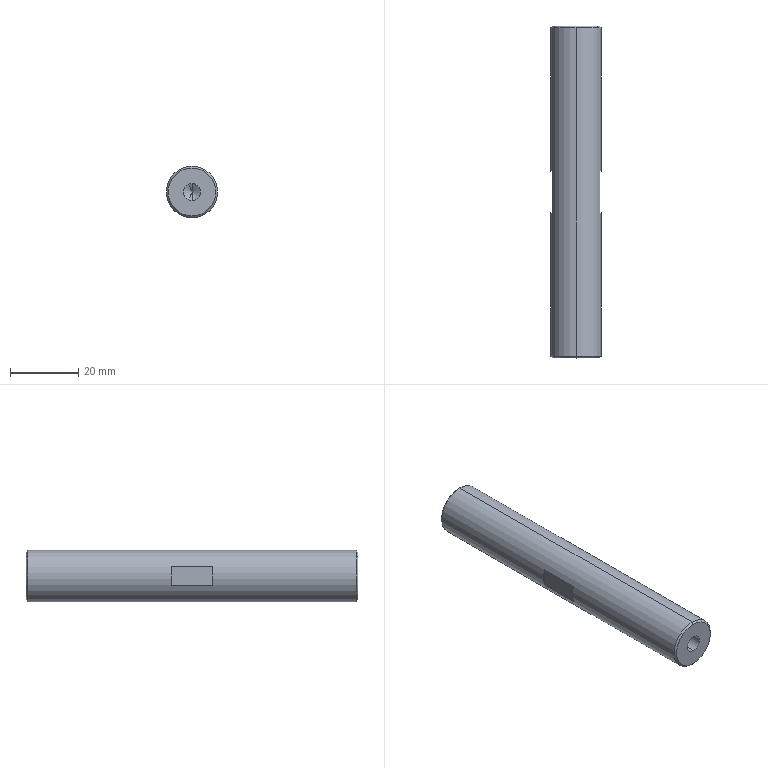Part | STEP file | ND25021-01-JDKM-40-TL | 1 solid | 22 faces | box 15 x 97 x 15 mm | volume 16574 mm3 | cone 8 | plane 8 | cylinder 6 | commonest cylinder face diameters 5 x4 15 x2
STEP:
#1=CARTESIAN_POINT('',(0.,0.,0.));
#2=DIRECTION('',(0.,0.,1.));
#3=DIRECTION('',(1.,0.,0.));
#4=AXIS2_PLACEMENT_3D('',#1,#2,#3);
#5=CARTESIAN_POINT('',(0.,82.,2.5));
#6=VERTEX_POINT('',#5);
#7=CARTESIAN_POINT('',(0.,97.,2.5));
#8=VERTEX_POINT('',#7);
#9=CARTESIAN_POINT('',(0.,97.,2.5));
#10=DIRECTION('',(0.,1.,0.));
#11=VECTOR('',#10,1.);
#12=LINE('',#9,#11);
#13=CARTESIAN_POINT('',(0.,97.,0.));
#14=DIRECTION('',(0.,1.,0.));
#15=DIRECTION('',(0.,0.,1.));
#16=AXIS2_PLACEMENT_3D('',#13,#14,#15);
#17=CYLINDRICAL_SURFACE('',#16,2.5);
#18=CARTESIAN_POINT('',(6.283,0.));
#19=DIRECTION('',(0.,1.));
#20=VECTOR('',#19,1.);
#21=LINE('',#18,#20);
#22=(GEOMETRIC_REPRESENTATION_CONTEXT(2)PARAMETRIC_REPRESENTATION_CONTEXT()REPRESENTATION_CONTEXT('',''));
#23=DEFINITIONAL_REPRESENTATION('',(#21),#22);
#24=PCURVE('',#17,#23);
#25=CARTESIAN_POINT('',(0.,97.,0.));
#26=DIRECTION('',(0.,1.,0.));
#27=DIRECTION('',(0.,0.,1.));
#28=AXIS2_PLACEMENT_3D('',#25,#26,#27);
#29=CYLINDRICAL_SURFACE('',#28,2.5);
#30=CARTESIAN_POINT('',(0.,0.));
#31=DIRECTION('',(0.,1.));
#32=VECTOR('',#31,1.);
#33=LINE('',#30,#32);
#34=(GEOMETRIC_REPRESENTATION_CONTEXT(2)PARAMETRIC_REPRESENTATION_CONTEXT()REPRESENTATION_CONTEXT('',''));
#35=DEFINITIONAL_REPRESENTATION('',(#33),#34);
#36=PCURVE('',#29,#35);
#37=SURFACE_CURVE('',#12,(#24,#36),.PCURVE_S1.);
#38=EDGE_CURVE('',#6,#8,#37,.T.);
#39=ORIENTED_EDGE('',*,*,#38,.T.);
#40=CARTESIAN_POINT('',(0.,97.,-2.5));
#41=VERTEX_POINT('',#40);
#42=CARTESIAN_POINT('',(0.,97.,0.));
#43=DIRECTION('',(0.,1.,0.));
#44=DIRECTION('',(0.,0.,1.));
#45=AXIS2_PLACEMENT_3D('',#42,#43,#44);
#46=CIRCLE('',#45,2.5);
#47=CARTESIAN_POINT('',(0.,0.));
#48=DIRECTION('',(1.,0.));
#49=VECTOR('',#48,1.);
#50=LINE('',#47,#49);
#51=(GEOMETRIC_REPRESENTATION_CONTEXT(2)PARAMETRIC_REPRESENTATION_CONTEXT()REPRESENTATION_CONTEXT('',''));
#52=DEFINITIONAL_REPRESENTATION('',(#50),#51);
#53=PCURVE('',#17,#52);
#54=CARTESIAN_POINT('',(0.,97.,0.));
#55=DIRECTION('',(0.,1.,0.));
#56=DIRECTION('',(0.,0.,1.));
#57=AXIS2_PLACEMENT_3D('',#54,#55,#56);
#58=PLANE('',#57);
#59=CARTESIAN_POINT('',(0.,0.));
#60=DIRECTION('',(1.,0.));
#61=AXIS2_PLACEMENT_2D('',#59,#60);
#62=CIRCLE('',#61,2.5);
#63=(GEOMETRIC_REPRESENTATION_CONTEXT(2)PARAMETRIC_REPRESENTATION_CONTEXT()REPRESENTATION_CONTEXT('',''));
#64=DEFINITIONAL_REPRESENTATION('',(#62),#63);
#65=PCURVE('',#58,#64);
#66=SURFACE_CURVE('',#46,(#53,#65),.PCURVE_S1.);
#67=EDGE_CURVE('',#41,#8,#66,.T.);
#68=ORIENTED_EDGE('',*,*,#67,.F.);
#69=CARTESIAN_POINT('',(0.,82.,-2.5));
#70=VERTEX_POINT('',#69);
#71=CARTESIAN_POINT('',(0.,97.,-2.5));
#72=DIRECTION('',(0.,1.,0.));
#73=VECTOR('',#72,1.);
#74=LINE('',#71,#73);
#75=CARTESIAN_POINT('',(3.142,0.));
#76=DIRECTION('',(0.,1.));
#77=VECTOR('',#76,1.);
#78=LINE('',#75,#77);
#79=(GEOMETRIC_REPRESENTATION_CONTEXT(2)PARAMETRIC_REPRESENTATION_CONTEXT()REPRESENTATION_CONTEXT('',''));
#80=DEFINITIONAL_REPRESENTATION('',(#78),#79);
#81=PCURVE('',#17,#80);
#82=CARTESIAN_POINT('',(3.142,0.));
#83=DIRECTION('',(0.,1.));
#84=VECTOR('',#83,1.);
#85=LINE('',#82,#84);
#86=(GEOMETRIC_REPRESENTATION_CONTEXT(2)PARAMETRIC_REPRESENTATION_CONTEXT()REPRESENTATION_CONTEXT('',''));
#87=DEFINITIONAL_REPRESENTATION('',(#85),#86);
#88=PCURVE('',#29,#87);
#89=SURFACE_CURVE('',#74,(#81,#88),.PCURVE_S1.);
#90=EDGE_CURVE('',#70,#41,#89,.T.);
#91=ORIENTED_EDGE('',*,*,#90,.F.);
#92=CARTESIAN_POINT('',(0.,82.,0.));
#93=DIRECTION('',(0.,1.,0.));
#94=DIRECTION('',(0.,0.,1.));
#95=AXIS2_PLACEMENT_3D('',#92,#93,#94);
#96=CIRCLE('',#95,2.5);
#97=CARTESIAN_POINT('',(0.,-15.));
#98=DIRECTION('',(1.,0.));
#99=VECTOR('',#98,1.);
#100=LINE('',#97,#99);
#101=(GEOMETRIC_REPRESENTATION_CONTEXT(2)PARAMETRIC_REPRESENTATION_CONTEXT()REPRESENTATION_CONTEXT('',''));
#102=DEFINITIONAL_REPRESENTATION('',(#100),#101);
#103=PCURVE('',#17,#102);
#104=CARTESIAN_POINT('',(0.,82.,0.));
#105=DIRECTION('',(0.,1.,0.));
#106=DIRECTION('',(0.,0.,1.));
#107=AXIS2_PLACEMENT_3D('',#104,#105,#106);
#108=CONICAL_SURFACE('',#107,2.5,1.03);
#109=CARTESIAN_POINT('',(0.,0.));
#110=DIRECTION('',(1.,0.));
#111=VECTOR('',#110,1.);
#112=LINE('',#109,#111);
#113=(GEOMETRIC_REPRESENTATION_CONTEXT(2)PARAMETRIC_REPRESENTATION_CONTEXT()REPRESENTATION_CONTEXT('',''));
#114=DEFINITIONAL_REPRESENTATION('',(#112),#113);
#115=PCURVE('',#108,#114);
#116=SURFACE_CURVE('',#96,(#103,#115),.PCURVE_S1.);
#117=EDGE_CURVE('',#70,#6,#116,.T.);
#118=ORIENTED_EDGE('',*,*,#117,.T.);
#119=EDGE_LOOP('',(#39,#68,#91,#118));
#120=FACE_BOUND('',#119,.F.);
#121=ADVANCED_FACE('',(#120),#17,.F.);
#122=ORIENTED_EDGE('',*,*,#117,.F.);
#123=CARTESIAN_POINT('',(0.,80.498,0.));
#124=VERTEX_POINT('',#123);
#125=CARTESIAN_POINT('',(0.,82.,-2.5));
#126=DIRECTION('',(0.,0.515,-0.8572));
#127=VECTOR('',#126,1.);
#128=LINE('',#125,#127);
#129=CARTESIAN_POINT('',(3.142,0.));
#130=DIRECTION('',(0.,1.));
#131=VECTOR('',#130,1.);
#132=LINE('',#129,#131);
#133=(GEOMETRIC_REPRESENTATION_CONTEXT(2)PARAMETRIC_REPRESENTATION_CONTEXT()REPRESENTATION_CONTEXT('',''));
#134=DEFINITIONAL_REPRESENTATION('',(#132),#133);
#135=PCURVE('',#108,#134);
#136=CARTESIAN_POINT('',(0.,82.,0.));
#137=DIRECTION('',(0.,1.,0.));
#138=DIRECTION('',(0.,0.,1.));
#139=AXIS2_PLACEMENT_3D('',#136,#137,#138);
#140=CONICAL_SURFACE('',#139,2.5,1.03);
#141=CARTESIAN_POINT('',(3.142,0.));
#142=DIRECTION('',(0.,1.));
#143=VECTOR('',#142,1.);
#144=LINE('',#141,#143);
#145=(GEOMETRIC_REPRESENTATION_CONTEXT(2)PARAMETRIC_REPRESENTATION_CONTEXT()REPRESENTATION_CONTEXT('',''));
#146=DEFINITIONAL_REPRESENTATION('',(#144),#145);
#147=PCURVE('',#140,#146);
#148=SURFACE_CURVE('',#128,(#135,#147),.PCURVE_S1.);
#149=EDGE_CURVE('',#124,#70,#148,.T.);
#150=ORIENTED_EDGE('',*,*,#149,.F.);
#151=CARTESIAN_POINT('',(0.,82.,2.5));
#152=DIRECTION('',(0.,0.515,0.8572));
#153=VECTOR('',#152,1.);
#154=LINE('',#151,#153);
#155=CARTESIAN_POINT('',(6.283,0.));
#156=DIRECTION('',(0.,1.));
#157=VECTOR('',#156,1.);
#158=LINE('',#155,#157);
#159=(GEOMETRIC_REPRESENTATION_CONTEXT(2)PARAMETRIC_REPRESENTATION_CONTEXT()REPRESENTATION_CONTEXT('',''));
#160=DEFINITIONAL_REPRESENTATION('',(#158),#159);
#161=PCURVE('',#108,#160);
#162=CARTESIAN_POINT('',(0.,0.));
#163=DIRECTION('',(0.,1.));
#164=VECTOR('',#163,1.);
#165=LINE('',#162,#164);
#166=(GEOMETRIC_REPRESENTATION_CONTEXT(2)PARAMETRIC_REPRESENTATION_CONTEXT()REPRESENTATION_CONTEXT('',''));
#167=DEFINITIONAL_REPRESENTATION('',(#165),#166);
#168=PCURVE('',#140,#167);
#169=SURFACE_CURVE('',#154,(#161,#168),.PCURVE_S1.);
#170=EDGE_CURVE('',#124,#6,#169,.T.);
#171=ORIENTED_EDGE('',*,*,#170,.T.);
#172=EDGE_LOOP('',(#122,#150,#171));
#173=FACE_BOUND('',#172,.F.);
#174=ADVANCED_FACE('',(#173),#108,.F.);
#175=CARTESIAN_POINT('',(0.,10.1,-2.5));
#176=VERTEX_POINT('',#175);
#177=CARTESIAN_POINT('',(0.,0.,-2.5));
#178=VERTEX_POINT('',#177);
#179=CARTESIAN_POINT('',(0.,0.,-2.5));
#180=DIRECTION('',(0.,-1.,0.));
#181=VECTOR('',#180,1.);
#182=LINE('',#179,#181);
#183=CARTESIAN_POINT('',(0.,0.,0.));
#184=DIRECTION('',(0.,-1.,0.));
#185=DIRECTION('',(0.,0.,-1.));
#186=AXIS2_PLACEMENT_3D('',#183,#184,#185);
#187=CYLINDRICAL_SURFACE('',#186,2.5);
#188=CARTESIAN_POINT('',(6.283,0.));
#189=DIRECTION('',(0.,1.));
#190=VECTOR('',#189,1.);
#191=LINE('',#188,#190);
#192=(GEOMETRIC_REPRESENTATION_CONTEXT(2)PARAMETRIC_REPRESENTATION_CONTEXT()REPRESENTATION_CONTEXT('',''));
#193=DEFINITIONAL_REPRESENTATION('',(#191),#192);
#194=PCURVE('',#187,#193);
#195=CARTESIAN_POINT('',(0.,0.,0.));
#196=DIRECTION('',(0.,-1.,0.));
#197=DIRECTION('',(0.,0.,-1.));
#198=AXIS2_PLACEMENT_3D('',#195,#196,#197);
#199=CYLINDRICAL_SURFACE('',#198,2.5);
#200=CARTESIAN_POINT('',(0.,0.));
#201=DIRECTION('',(0.,1.));
#202=VECTOR('',#201,1.);
#203=LINE('',#200,#202);
#204=(GEOMETRIC_REPRESENTATION_CONTEXT(2)PARAMETRIC_REPRESENTATION_CONTEXT()REPRESENTATION_CONTEXT('',''));
#205=DEFINITIONAL_REPRESENTATION('',(#203),#204);
#206=PCURVE('',#199,#205);
#207=SURFACE_CURVE('',#182,(#194,#206),.PCURVE_S1.);
#208=EDGE_CURVE('',#176,#178,#207,.T.);
#209=ORIENTED_EDGE('',*,*,#208,.T.);
#210=CARTESIAN_POINT('',(0.,0.,2.5));
#211=VERTEX_POINT('',#210);
#212=CARTESIAN_POINT('',(0.,0.,0.));
#213=DIRECTION('',(0.,-1.,0.));
#214=DIRECTION('',(0.,0.,-1.));
#215=AXIS2_PLACEMENT_3D('',#212,#213,#214);
#216=CIRCLE('',#215,2.5);
#217=CARTESIAN_POINT('',(0.,0.));
#218=DIRECTION('',(1.,0.));
#219=VECTOR('',#218,1.);
#220=LINE('',#217,#219);
#221=(GEOMETRIC_REPRESENTATION_CONTEXT(2)PARAMETRIC_REPRESENTATION_CONTEXT()REPRESENTATION_CONTEXT('',''));
#222=DEFINITIONAL_REPRESENTATION('',(#220),#221);
#223=PCURVE('',#187,#222);
#224=CARTESIAN_POINT('',(0.,0.,0.));
#225=DIRECTION('',(0.,1.,0.));
#226=DIRECTION('',(0.,0.,1.));
#227=AXIS2_PLACEMENT_3D('',#224,#225,#226);
#228=PLANE('',#227);
#229=CARTESIAN_POINT('',(-2.5,0.));
#230=CARTESIAN_POINT('',(-2.5,4.33));
#231=CARTESIAN_POINT('',(1.25,2.165));
#232=CARTESIAN_POINT('',(5.,0.));
#233=CARTESIAN_POINT('',(1.25,-2.165));
#234=CARTESIAN_POINT('',(-2.5,-4.33));
#235=CARTESIAN_POINT('',(-2.5,0.));
#236=(BOUNDED_CURVE()B_SPLINE_CURVE(2,(#229,#230,#231,#232,#233,#234,#235),.UNSPECIFIED.,.T.,.F.)B_SPLINE_CURVE_WITH_KNOTS((1,2,2,2,2,1),(-2.094,0.,2.094,4.189,6.283,8.378),.UNSPECIFIED.)CURVE()GEOMETRIC_REPRESENTATION_ITEM()RATIONAL_B_SPLINE_CURVE((1.,0.5,1.,0.5,1.,0.5,1.))REPRESENTATION_ITEM(''));
#237=(GEOMETRIC_REPRESENTATION_CONTEXT(2)PARAMETRIC_REPRESENTATION_CONTEXT()REPRESENTATION_CONTEXT('',''));
#238=DEFINITIONAL_REPRESENTATION('',(#236),#237);
#239=PCURVE('',#228,#238);
#240=SURFACE_CURVE('',#216,(#223,#239),.PCURVE_S1.);
#241=EDGE_CURVE('',#211,#178,#240,.T.);
#242=ORIENTED_EDGE('',*,*,#241,.F.);
#243=CARTESIAN_POINT('',(0.,10.1,2.5));
#244=VERTEX_POINT('',#243);
#245=CARTESIAN_POINT('',(0.,0.,2.5));
#246=DIRECTION('',(0.,-1.,0.));
#247=VECTOR('',#246,1.);
#248=LINE('',#245,#247);
#249=CARTESIAN_POINT('',(3.142,0.));
#250=DIRECTION('',(0.,1.));
#251=VECTOR('',#250,1.);
#252=LINE('',#249,#251);
#253=(GEOMETRIC_REPRESENTATION_CONTEXT(2)PARAMETRIC_REPRESENTATION_CONTEXT()REPRESENTATION_CONTEXT('',''));
#254=DEFINITIONAL_REPRESENTATION('',(#252),#253);
#255=PCURVE('',#187,#254);
#256=CARTESIAN_POINT('',(3.142,0.));
#257=DIRECTION('',(0.,1.));
#258=VECTOR('',#257,1.);
#259=LINE('',#256,#258);
#260=(GEOMETRIC_REPRESENTATION_CONTEXT(2)PARAMETRIC_REPRESENTATION_CONTEXT()REPRESENTATION_CONTEXT('',''));
#261=DEFINITIONAL_REPRESENTATION('',(#259),#260);
#262=PCURVE('',#199,#261);
#263=SURFACE_CURVE('',#248,(#255,#262),.PCURVE_S1.);
#264=EDGE_CURVE('',#244,#211,#263,.T.);
#265=ORIENTED_EDGE('',*,*,#264,.F.);
#266=CARTESIAN_POINT('',(0.,10.1,0.));
#267=DIRECTION('',(0.,-1.,0.));
#268=DIRECTION('',(0.,0.,-1.));
#269=AXIS2_PLACEMENT_3D('',#266,#267,#268);
#270=CIRCLE('',#269,2.5);
#271=CARTESIAN_POINT('',(0.,-10.1));
#272=DIRECTION('',(1.,0.));
#273=VECTOR('',#272,1.);
#274=LINE('',#271,#273);
#275=(GEOMETRIC_REPRESENTATION_CONTEXT(2)PARAMETRIC_REPRESENTATION_CONTEXT()REPRESENTATION_CONTEXT('',''));
#276=DEFINITIONAL_REPRESENTATION('',(#274),#275);
#277=PCURVE('',#187,#276);
#278=CARTESIAN_POINT('',(0.,10.1,0.));
#279=DIRECTION('',(0.,-1.,0.));
#280=DIRECTION('',(0.,0.,-1.));
#281=AXIS2_PLACEMENT_3D('',#278,#279,#280);
#282=CONICAL_SURFACE('',#281,2.5,1.03);
#283=CARTESIAN_POINT('',(0.,0.));
#284=DIRECTION('',(1.,0.));
#285=VECTOR('',#284,1.);
#286=LINE('',#283,#285);
#287=(GEOMETRIC_REPRESENTATION_CONTEXT(2)PARAMETRIC_REPRESENTATION_CONTEXT()REPRESENTATION_CONTEXT('',''));
#288=DEFINITIONAL_REPRESENTATION('',(#286),#287);
#289=PCURVE('',#282,#288);
#290=SURFACE_CURVE('',#270,(#277,#289),.PCURVE_S1.);
#291=EDGE_CURVE('',#244,#176,#290,.T.);
#292=ORIENTED_EDGE('',*,*,#291,.T.);
#293=EDGE_LOOP('',(#209,#242,#265,#292));
#294=FACE_BOUND('',#293,.F.);
#295=ADVANCED_FACE('',(#294),#187,.F.);
#296=ORIENTED_EDGE('',*,*,#291,.F.);
#297=CARTESIAN_POINT('',(0.,11.602,0.));
#298=VERTEX_POINT('',#297);
#299=CARTESIAN_POINT('',(0.,10.1,2.5));
#300=DIRECTION('',(0.,-0.515,0.8572));
#301=VECTOR('',#300,1.);
#302=LINE('',#299,#301);
#303=CARTESIAN_POINT('',(3.142,-1.502));
#304=CARTESIAN_POINT('',(3.142,-1.479));
#305=CARTESIAN_POINT('',(3.142,-1.434));
#306=CARTESIAN_POINT('',(3.142,-1.366));
#307=CARTESIAN_POINT('',(3.142,-1.297));
#308=CARTESIAN_POINT('',(3.142,-1.229));
#309=CARTESIAN_POINT('',(3.142,-1.161));
#310=CARTESIAN_POINT('',(3.142,-1.092));
#311=CARTESIAN_POINT('',(3.142,-1.024));
#312=CARTESIAN_POINT('',(3.142,-0.9559));
#313=CARTESIAN_POINT('',(3.142,-0.8876));
#314=CARTESIAN_POINT('',(3.142,-0.8194));
#315=CARTESIAN_POINT('',(3.142,-0.7511));
#316=CARTESIAN_POINT('',(3.142,-0.6828));
#317=CARTESIAN_POINT('',(3.142,-0.6145));
#318=CARTESIAN_POINT('',(3.142,-0.5462));
#319=CARTESIAN_POINT('',(3.142,-0.478));
#320=CARTESIAN_POINT('',(3.142,-0.4097));
#321=CARTESIAN_POINT('',(3.142,-0.3414));
#322=CARTESIAN_POINT('',(3.142,-0.2731));
#323=CARTESIAN_POINT('',(3.142,-0.2048));
#324=CARTESIAN_POINT('',(3.142,-0.1366));
#325=CARTESIAN_POINT('',(3.142,-0.06828));
#326=CARTESIAN_POINT('',(3.142,-0.02276));
#327=CARTESIAN_POINT('',(3.142,0.));
#328=B_SPLINE_CURVE_WITH_KNOTS('',3,(#303,#304,#305,#306,#307,#308,#309,#310,#311,#312,#313,#314,#315,#316,#317,#318,#319,#320,#321,#322,#323,#324,#325,#326,#327),.UNSPECIFIED.,.F.,.F.,(4,1,1,1,1,1,1,1,1,1,1,1,1,1,1,1,1,1,1,1,1,1,4),(-2.917,-2.784,-2.651,-2.519,-2.386,-2.254,-2.121,-1.989,-1.856,-1.723,-1.591,-1.458,-1.326,-1.193,-1.061,-0.928,-0.7954,-0.6629,-0.5303,-0.3977,-0.2651,-0.1326,0.),.UNSPECIFIED.);
#329=(GEOMETRIC_REPRESENTATION_CONTEXT(2)PARAMETRIC_REPRESENTATION_CONTEXT()REPRESENTATION_CONTEXT('',''));
#330=DEFINITIONAL_REPRESENTATION('',(#328),#329);
#331=PCURVE('',#282,#330);
#332=CARTESIAN_POINT('',(0.,10.1,0.));
#333=DIRECTION('',(0.,-1.,0.));
#334=DIRECTION('',(0.,0.,-1.));
#335=AXIS2_PLACEMENT_3D('',#332,#333,#334);
#336=CONICAL_SURFACE('',#335,2.5,1.03);
#337=CARTESIAN_POINT('',(3.142,-1.502));
#338=CARTESIAN_POINT('',(3.142,-1.479));
#339=CARTESIAN_POINT('',(3.142,-1.434));
#340=CARTESIAN_POINT('',(3.142,-1.366));
#341=CARTESIAN_POINT('',(3.142,-1.297));
#342=CARTESIAN_POINT('',(3.142,-1.229));
#343=CARTESIAN_POINT('',(3.142,-1.161));
#344=CARTESIAN_POINT('',(3.142,-1.092));
#345=CARTESIAN_POINT('',(3.142,-1.024));
#346=CARTESIAN_POINT('',(3.142,-0.9559));
#347=CARTESIAN_POINT('',(3.142,-0.8876));
#348=CARTESIAN_POINT('',(3.142,-0.8194));
#349=CARTESIAN_POINT('',(3.142,-0.7511));
#350=CARTESIAN_POINT('',(3.142,-0.6828));
#351=CARTESIAN_POINT('',(3.142,-0.6145));
#352=CARTESIAN_POINT('',(3.142,-0.5462));
#353=CARTESIAN_POINT('',(3.142,-0.478));
#354=CARTESIAN_POINT('',(3.142,-0.4097));
#355=CARTESIAN_POINT('',(3.142,-0.3414));
#356=CARTESIAN_POINT('',(3.142,-0.2731));
#357=CARTESIAN_POINT('',(3.142,-0.2048));
#358=CARTESIAN_POINT('',(3.142,-0.1366));
#359=CARTESIAN_POINT('',(3.142,-0.06828));
#360=CARTESIAN_POINT('',(3.142,-0.02276));
#361=CARTESIAN_POINT('',(3.142,0.));
#362=B_SPLINE_CURVE_WITH_KNOTS('',3,(#337,#338,#339,#340,#341,#342,#343,#344,#345,#346,#347,#348,#349,#350,#351,#352,#353,#354,#355,#356,#357,#358,#359,#360,#361),.UNSPECIFIED.,.F.,.F.,(4,1,1,1,1,1,1,1,1,1,1,1,1,1,1,1,1,1,1,1,1,1,4),(-2.917,-2.784,-2.651,-2.519,-2.386,-2.254,-2.121,-1.989,-1.856,-1.723,-1.591,-1.458,-1.326,-1.193,-1.061,-0.928,-0.7954,-0.6629,-0.5303,-0.3977,-0.2651,-0.1326,0.),.UNSPECIFIED.);
#363=(GEOMETRIC_REPRESENTATION_CONTEXT(2)PARAMETRIC_REPRESENTATION_CONTEXT()REPRESENTATION_CONTEXT('',''));
#364=DEFINITIONAL_REPRESENTATION('',(#362),#363);
#365=PCURVE('',#336,#364);
#366=SURFACE_CURVE('',#302,(#331,#365),.PCURVE_S1.);
#367=EDGE_CURVE('',#298,#244,#366,.T.);
#368=ORIENTED_EDGE('',*,*,#367,.F.);
#369=CARTESIAN_POINT('',(0.,10.1,-2.5));
#370=DIRECTION('',(0.,-0.515,-0.8572));
#371=VECTOR('',#370,1.);
#372=LINE('',#369,#371);
#373=CARTESIAN_POINT('',(6.283,-1.502));
#374=CARTESIAN_POINT('',(6.283,-1.479));
#375=CARTESIAN_POINT('',(6.283,-1.434));
#376=CARTESIAN_POINT('',(6.283,-1.366));
#377=CARTESIAN_POINT('',(6.283,-1.297));
#378=CARTESIAN_POINT('',(6.283,-1.229));
#379=CARTESIAN_POINT('',(6.283,-1.161));
#380=CARTESIAN_POINT('',(6.283,-1.092));
#381=CARTESIAN_POINT('',(6.283,-1.024));
#382=CARTESIAN_POINT('',(6.283,-0.9559));
#383=CARTESIAN_POINT('',(6.283,-0.8876));
#384=CARTESIAN_POINT('',(6.283,-0.8194));
#385=CARTESIAN_POINT('',(6.283,-0.7511));
#386=CARTESIAN_POINT('',(6.283,-0.6828));
#387=CARTESIAN_POINT('',(6.283,-0.6145));
#388=CARTESIAN_POINT('',(6.283,-0.5462));
#389=CARTESIAN_POINT('',(6.283,-0.478));
#390=CARTESIAN_POINT('',(6.283,-0.4097));
#391=CARTESIAN_POINT('',(6.283,-0.3414));
#392=CARTESIAN_POINT('',(6.283,-0.2731));
#393=CARTESIAN_POINT('',(6.283,-0.2048));
#394=CARTESIAN_POINT('',(6.283,-0.1366));
#395=CARTESIAN_POINT('',(6.283,-0.06828));
#396=CARTESIAN_POINT('',(6.283,-0.02276));
#397=CARTESIAN_POINT('',(6.283,0.));
#398=B_SPLINE_CURVE_WITH_KNOTS('',3,(#373,#374,#375,#376,#377,#378,#379,#380,#381,#382,#383,#384,#385,#386,#387,#388,#389,#390,#391,#392,#393,#394,#395,#396,#397),.UNSPECIFIED.,.F.,.F.,(4,1,1,1,1,1,1,1,1,1,1,1,1,1,1,1,1,1,1,1,1,1,4),(-2.917,-2.784,-2.651,-2.519,-2.386,-2.254,-2.121,-1.989,-1.856,-1.723,-1.591,-1.458,-1.326,-1.193,-1.061,-0.928,-0.7954,-0.6629,-0.5303,-0.3977,-0.2651,-0.1326,0.),.UNSPECIFIED.);
#399=(GEOMETRIC_REPRESENTATION_CONTEXT(2)PARAMETRIC_REPRESENTATION_CONTEXT()REPRESENTATION_CONTEXT('',''));
#400=DEFINITIONAL_REPRESENTATION('',(#398),#399);
#401=PCURVE('',#282,#400);
#402=CARTESIAN_POINT('',(0.,-1.502));
#403=CARTESIAN_POINT('',(0.,-1.479));
#404=CARTESIAN_POINT('',(0.,-1.434));
#405=CARTESIAN_POINT('',(0.,-1.366));
#406=CARTESIAN_POINT('',(0.,-1.297));
#407=CARTESIAN_POINT('',(0.,-1.229));
#408=CARTESIAN_POINT('',(0.,-1.161));
#409=CARTESIAN_POINT('',(0.,-1.092));
#410=CARTESIAN_POINT('',(0.,-1.024));
#411=CARTESIAN_POINT('',(0.,-0.9559));
#412=CARTESIAN_POINT('',(0.,-0.8876));
#413=CARTESIAN_POINT('',(0.,-0.8194));
#414=CARTESIAN_POINT('',(0.,-0.7511));
#415=CARTESIAN_POINT('',(0.,-0.6828));
#416=CARTESIAN_POINT('',(0.,-0.6145));
#417=CARTESIAN_POINT('',(0.,-0.5462));
#418=CARTESIAN_POINT('',(0.,-0.478));
#419=CARTESIAN_POINT('',(0.,-0.4097));
#420=CARTESIAN_POINT('',(0.,-0.3414));
#421=CARTESIAN_POINT('',(0.,-0.2731));
#422=CARTESIAN_POINT('',(0.,-0.2048));
#423=CARTESIAN_POINT('',(0.,-0.1366));
#424=CARTESIAN_POINT('',(0.,-0.06828));
#425=CARTESIAN_POINT('',(0.,-0.02276));
#426=CARTESIAN_POINT('',(0.,0.));
#427=B_SPLINE_CURVE_WITH_KNOTS('',3,(#402,#403,#404,#405,#406,#407,#408,#409,#410,#411,#412,#413,#414,#415,#416,#417,#418,#419,#420,#421,#422,#423,#424,#425,#426),.UNSPECIFIED.,.F.,.F.,(4,1,1,1,1,1,1,1,1,1,1,1,1,1,1,1,1,1,1,1,1,1,4),(-2.917,-2.784,-2.651,-2.519,-2.386,-2.254,-2.121,-1.989,-1.856,-1.723,-1.591,-1.458,-1.326,-1.193,-1.061,-0.928,-0.7954,-0.6629,-0.5303,-0.3977,-0.2651,-0.1326,0.),.UNSPECIFIED.);
#428=(GEOMETRIC_REPRESENTATION_CONTEXT(2)PARAMETRIC_REPRESENTATION_CONTEXT()REPRESENTATION_CONTEXT('',''));
#429=DEFINITIONAL_REPRESENTATION('',(#427),#428);
#430=PCURVE('',#336,#429);
#431=SURFACE_CURVE('',#372,(#401,#430),.PCURVE_S1.);
#432=EDGE_CURVE('',#298,#176,#431,.T.);
#433=ORIENTED_EDGE('',*,*,#432,.T.);
#434=EDGE_LOOP('',(#296,#368,#433));
#435=FACE_BOUND('',#434,.F.);
#436=ADVANCED_FACE('',(#435),#282,.F.);
#437=CARTESIAN_POINT('',(0.,97.,7.));
#438=VERTEX_POINT('',#437);
#439=CARTESIAN_POINT('',(0.,97.,-7.));
#440=VERTEX_POINT('',#439);
#441=CARTESIAN_POINT('',(0.,97.,0.));
#442=DIRECTION('',(0.,1.,0.));
#443=DIRECTION('',(0.,0.,1.));
#444=AXIS2_PLACEMENT_3D('',#441,#442,#443);
#445=CIRCLE('',#444,7.);
#446=CARTESIAN_POINT('',(0.,97.,0.));
#447=DIRECTION('',(0.,-1.,0.));
#448=DIRECTION('',(0.,0.,-1.));
#449=AXIS2_PLACEMENT_3D('',#446,#447,#448);
#450=CONICAL_SURFACE('',#449,7.,0.7854);
#451=CARTESIAN_POINT('',(3.142,0.));
#452=DIRECTION('',(-1.,0.));
#453=VECTOR('',#452,1.);
#454=LINE('',#451,#453);
#455=(GEOMETRIC_REPRESENTATION_CONTEXT(2)PARAMETRIC_REPRESENTATION_CONTEXT()REPRESENTATION_CONTEXT('',''));
#456=DEFINITIONAL_REPRESENTATION('',(#454),#455);
#457=PCURVE('',#450,#456);
#458=CARTESIAN_POINT('',(0.,0.));
#459=DIRECTION('',(1.,0.));
#460=AXIS2_PLACEMENT_2D('',#458,#459);
#461=CIRCLE('',#460,7.);
#462=(GEOMETRIC_REPRESENTATION_CONTEXT(2)PARAMETRIC_REPRESENTATION_CONTEXT()REPRESENTATION_CONTEXT('',''));
#463=DEFINITIONAL_REPRESENTATION('',(#461),#462);
#464=PCURVE('',#58,#463);
#465=SURFACE_CURVE('',#445,(#457,#464),.PCURVE_S1.);
#466=EDGE_CURVE('',#438,#440,#465,.T.);
#467=ORIENTED_EDGE('',*,*,#466,.F.);
#468=CARTESIAN_POINT('',(0.,96.5,7.5));
#469=VERTEX_POINT('',#468);
#470=CARTESIAN_POINT('',(0.,97.,7.));
#471=DIRECTION('',(0.,-0.7071,0.7071));
#472=VECTOR('',#471,1.);
#473=LINE('',#470,#472);
#474=CARTESIAN_POINT('',(3.142,0.));
#475=DIRECTION('',(0.,1.));
#476=VECTOR('',#475,1.);
#477=LINE('',#474,#476);
#478=(GEOMETRIC_REPRESENTATION_CONTEXT(2)PARAMETRIC_REPRESENTATION_CONTEXT()REPRESENTATION_CONTEXT('',''));
#479=DEFINITIONAL_REPRESENTATION('',(#477),#478);
#480=PCURVE('',#450,#479);
#481=CARTESIAN_POINT('',(0.,97.,0.));
#482=DIRECTION('',(0.,-1.,0.));
#483=DIRECTION('',(0.,0.,-1.));
#484=AXIS2_PLACEMENT_3D('',#481,#482,#483);
#485=CONICAL_SURFACE('',#484,7.,0.7854);
#486=CARTESIAN_POINT('',(3.142,0.));
#487=DIRECTION('',(0.,1.));
#488=VECTOR('',#487,1.);
#489=LINE('',#486,#488);
#490=(GEOMETRIC_REPRESENTATION_CONTEXT(2)PARAMETRIC_REPRESENTATION_CONTEXT()REPRESENTATION_CONTEXT('',''));
#491=DEFINITIONAL_REPRESENTATION('',(#489),#490);
#492=PCURVE('',#485,#491);
#493=SURFACE_CURVE('',#473,(#480,#492),.PCURVE_S1.);
#494=EDGE_CURVE('',#438,#469,#493,.T.);
#495=ORIENTED_EDGE('',*,*,#494,.T.);
#496=CARTESIAN_POINT('',(0.,96.5,-7.5));
#497=VERTEX_POINT('',#496);
#498=CARTESIAN_POINT('',(0.,96.5,0.));
#499=DIRECTION('',(0.,-1.,0.));
#500=DIRECTION('',(0.,0.,1.));
#501=AXIS2_PLACEMENT_3D('',#498,#499,#500);
#502=CIRCLE('',#501,7.5);
#503=CARTESIAN_POINT('',(-3.142,0.5));
#504=DIRECTION('',(1.,0.));
#505=VECTOR('',#504,1.);
#506=LINE('',#503,#505);
#507=(GEOMETRIC_REPRESENTATION_CONTEXT(2)PARAMETRIC_REPRESENTATION_CONTEXT()REPRESENTATION_CONTEXT('',''));
#508=DEFINITIONAL_REPRESENTATION('',(#506),#507);
#509=PCURVE('',#450,#508);
#510=CARTESIAN_POINT('',(0.,97.,0.));
#511=DIRECTION('',(0.,-1.,0.));
#512=DIRECTION('',(0.,0.,-1.));
#513=AXIS2_PLACEMENT_3D('',#510,#511,#512);
#514=CYLINDRICAL_SURFACE('',#513,7.5);
#515=CARTESIAN_POINT('',(-3.142,0.5));
#516=DIRECTION('',(1.,0.));
#517=VECTOR('',#516,1.);
#518=LINE('',#515,#517);
#519=(GEOMETRIC_REPRESENTATION_CONTEXT(2)PARAMETRIC_REPRESENTATION_CONTEXT()REPRESENTATION_CONTEXT('',''));
#520=DEFINITIONAL_REPRESENTATION('',(#518),#519);
#521=PCURVE('',#514,#520);
#522=SURFACE_CURVE('',#502,(#509,#521),.PCURVE_S1.);
#523=EDGE_CURVE('',#497,#469,#522,.T.);
#524=ORIENTED_EDGE('',*,*,#523,.F.);
#525=CARTESIAN_POINT('',(0.,97.,-7.));
#526=DIRECTION('',(0.,-0.7071,-0.7071));
#527=VECTOR('',#526,1.);
#528=LINE('',#525,#527);
#529=CARTESIAN_POINT('',(0.,0.));
#530=DIRECTION('',(0.,1.));
#531=VECTOR('',#530,1.);
#532=LINE('',#529,#531);
#533=(GEOMETRIC_REPRESENTATION_CONTEXT(2)PARAMETRIC_REPRESENTATION_CONTEXT()REPRESENTATION_CONTEXT('',''));
#534=DEFINITIONAL_REPRESENTATION('',(#532),#533);
#535=PCURVE('',#450,#534);
#536=CARTESIAN_POINT('',(6.283,0.));
#537=DIRECTION('',(0.,1.));
#538=VECTOR('',#537,1.);
#539=LINE('',#536,#538);
#540=(GEOMETRIC_REPRESENTATION_CONTEXT(2)PARAMETRIC_REPRESENTATION_CONTEXT()REPRESENTATION_CONTEXT('',''));
#541=DEFINITIONAL_REPRESENTATION('',(#539),#540);
#542=PCURVE('',#485,#541);
#543=SURFACE_CURVE('',#528,(#535,#542),.PCURVE_S1.);
#544=EDGE_CURVE('',#440,#497,#543,.T.);
#545=ORIENTED_EDGE('',*,*,#544,.F.);
#546=EDGE_LOOP('',(#467,#495,#524,#545));
#547=FACE_BOUND('',#546,.T.);
#548=ADVANCED_FACE('',(#547),#450,.T.);
#549=CARTESIAN_POINT('',(0.,0.,-7.));
#550=VERTEX_POINT('',#549);
#551=CARTESIAN_POINT('',(0.,0.,7.));
#552=VERTEX_POINT('',#551);
#553=CARTESIAN_POINT('',(0.,0.,0.));
#554=DIRECTION('',(0.,-1.,0.));
#555=DIRECTION('',(0.,0.,1.));
#556=AXIS2_PLACEMENT_3D('',#553,#554,#555);
#557=CIRCLE('',#556,7.);
#558=CARTESIAN_POINT('',(0.,0.5,0.));
#559=DIRECTION('',(0.,1.,0.));
#560=DIRECTION('',(0.,0.,1.));
#561=AXIS2_PLACEMENT_3D('',#558,#559,#560);
#562=CONICAL_SURFACE('',#561,7.5,0.7854);
#563=CARTESIAN_POINT('',(6.283,-0.5));
#564=DIRECTION('',(-1.,0.));
#565=VECTOR('',#564,1.);
#566=LINE('',#563,#565);
#567=(GEOMETRIC_REPRESENTATION_CONTEXT(2)PARAMETRIC_REPRESENTATION_CONTEXT()REPRESENTATION_CONTEXT('',''));
#568=DEFINITIONAL_REPRESENTATION('',(#566),#567);
#569=PCURVE('',#562,#568);
#570=CARTESIAN_POINT('',(7.,0.));
#571=CARTESIAN_POINT('',(7.,-12.124));
#572=CARTESIAN_POINT('',(-3.5,-6.062));
#573=CARTESIAN_POINT('',(-14.,0.));
#574=CARTESIAN_POINT('',(-3.5,6.062));
#575=CARTESIAN_POINT('',(7.,12.124));
#576=CARTESIAN_POINT('',(7.,0.));
#577=(BOUNDED_CURVE()B_SPLINE_CURVE(2,(#570,#571,#572,#573,#574,#575,#576),.UNSPECIFIED.,.T.,.F.)B_SPLINE_CURVE_WITH_KNOTS((1,2,2,2,2,1),(-2.094,0.,2.094,4.189,6.283,8.378),.UNSPECIFIED.)CURVE()GEOMETRIC_REPRESENTATION_ITEM()RATIONAL_B_SPLINE_CURVE((1.,0.5,1.,0.5,1.,0.5,1.))REPRESENTATION_ITEM(''));
#578=(GEOMETRIC_REPRESENTATION_CONTEXT(2)PARAMETRIC_REPRESENTATION_CONTEXT()REPRESENTATION_CONTEXT('',''));
#579=DEFINITIONAL_REPRESENTATION('',(#577),#578);
#580=PCURVE('',#228,#579);
#581=SURFACE_CURVE('',#557,(#569,#580),.PCURVE_S1.);
#582=EDGE_CURVE('',#550,#552,#581,.T.);
#583=ORIENTED_EDGE('',*,*,#582,.F.);
#584=CARTESIAN_POINT('',(0.,0.5,-7.5));
#585=VERTEX_POINT('',#584);
#586=CARTESIAN_POINT('',(0.,0.5,-7.5));
#587=DIRECTION('',(0.,0.7071,-0.7071));
#588=VECTOR('',#587,1.);
#589=LINE('',#586,#588);
#590=CARTESIAN_POINT('',(3.142,0.));
#591=DIRECTION('',(0.,1.));
#592=VECTOR('',#591,1.);
#593=LINE('',#590,#592);
#594=(GEOMETRIC_REPRESENTATION_CONTEXT(2)PARAMETRIC_REPRESENTATION_CONTEXT()REPRESENTATION_CONTEXT('',''));
#595=DEFINITIONAL_REPRESENTATION('',(#593),#594);
#596=PCURVE('',#562,#595);
#597=CARTESIAN_POINT('',(0.,0.5,0.));
#598=DIRECTION('',(0.,1.,0.));
#599=DIRECTION('',(0.,0.,1.));
#600=AXIS2_PLACEMENT_3D('',#597,#598,#599);
#601=CONICAL_SURFACE('',#600,7.5,0.7854);
#602=CARTESIAN_POINT('',(3.142,0.));
#603=DIRECTION('',(0.,1.));
#604=VECTOR('',#603,1.);
#605=LINE('',#602,#604);
#606=(GEOMETRIC_REPRESENTATION_CONTEXT(2)PARAMETRIC_REPRESENTATION_CONTEXT()REPRESENTATION_CONTEXT('',''));
#607=DEFINITIONAL_REPRESENTATION('',(#605),#606);
#608=PCURVE('',#601,#607);
#609=SURFACE_CURVE('',#589,(#596,#608),.PCURVE_S1.);
#610=EDGE_CURVE('',#550,#585,#609,.T.);
#611=ORIENTED_EDGE('',*,*,#610,.T.);
#612=CARTESIAN_POINT('',(0.,0.5,7.5));
#613=VERTEX_POINT('',#612);
#614=CARTESIAN_POINT('',(0.,0.5,0.));
#615=DIRECTION('',(0.,1.,0.));
#616=DIRECTION('',(0.,0.,1.));
#617=AXIS2_PLACEMENT_3D('',#614,#615,#616);
#618=CIRCLE('',#617,7.5);
#619=CARTESIAN_POINT('',(0.,0.));
#620=DIRECTION('',(1.,0.));
#621=VECTOR('',#620,1.);
#622=LINE('',#619,#621);
#623=(GEOMETRIC_REPRESENTATION_CONTEXT(2)PARAMETRIC_REPRESENTATION_CONTEXT()REPRESENTATION_CONTEXT('',''));
#624=DEFINITIONAL_REPRESENTATION('',(#622),#623);
#625=PCURVE('',#562,#624);
#626=CARTESIAN_POINT('',(3.142,96.5));
#627=DIRECTION('',(-1.,0.));
#628=VECTOR('',#627,1.);
#629=LINE('',#626,#628);
#630=(GEOMETRIC_REPRESENTATION_CONTEXT(2)PARAMETRIC_REPRESENTATION_CONTEXT()REPRESENTATION_CONTEXT('',''));
#631=DEFINITIONAL_REPRESENTATION('',(#629),#630);
#632=PCURVE('',#514,#631);
#633=SURFACE_CURVE('',#618,(#625,#632),.PCURVE_S1.);
#634=EDGE_CURVE('',#613,#585,#633,.T.);
#635=ORIENTED_EDGE('',*,*,#634,.F.);
#636=CARTESIAN_POINT('',(0.,0.5,7.5));
#637=DIRECTION('',(0.,0.7071,0.7071));
#638=VECTOR('',#637,1.);
#639=LINE('',#636,#638);
#640=CARTESIAN_POINT('',(0.,0.));
#641=DIRECTION('',(0.,1.));
#642=VECTOR('',#641,1.);
#643=LINE('',#640,#642);
#644=(GEOMETRIC_REPRESENTATION_CONTEXT(2)PARAMETRIC_REPRESENTATION_CONTEXT()REPRESENTATION_CONTEXT('',''));
#645=DEFINITIONAL_REPRESENTATION('',(#643),#644);
#646=PCURVE('',#562,#645);
#647=CARTESIAN_POINT('',(6.283,0.));
#648=DIRECTION('',(0.,1.));
#649=VECTOR('',#648,1.);
#650=LINE('',#647,#649);
#651=(GEOMETRIC_REPRESENTATION_CONTEXT(2)PARAMETRIC_REPRESENTATION_CONTEXT()REPRESENTATION_CONTEXT('',''));
#652=DEFINITIONAL_REPRESENTATION('',(#650),#651);
#653=PCURVE('',#601,#652);
#654=SURFACE_CURVE('',#639,(#646,#653),.PCURVE_S1.);
#655=EDGE_CURVE('',#552,#613,#654,.T.);
#656=ORIENTED_EDGE('',*,*,#655,.F.);
#657=EDGE_LOOP('',(#583,#611,#635,#656));
#658=FACE_BOUND('',#657,.T.);
#659=ADVANCED_FACE('',(#658),#562,.T.);
#660=CARTESIAN_POINT('',(7.,54.5,-2.693));
#661=VERTEX_POINT('',#660);
#662=CARTESIAN_POINT('',(7.,42.5,-2.693));
#663=VERTEX_POINT('',#662);
#664=CARTESIAN_POINT('',(7.,97.,-2.693));
#665=DIRECTION('',(0.,-1.,0.));
#666=VECTOR('',#665,1.);
#667=LINE('',#664,#666);
#668=CARTESIAN_POINT('',(1.204,0.));
#669=DIRECTION('',(0.,1.));
#670=VECTOR('',#669,1.);
#671=LINE('',#668,#670);
#672=(GEOMETRIC_REPRESENTATION_CONTEXT(2)PARAMETRIC_REPRESENTATION_CONTEXT()REPRESENTATION_CONTEXT('',''));
#673=DEFINITIONAL_REPRESENTATION('',(#671),#672);
#674=PCURVE('',#514,#673);
#675=CARTESIAN_POINT('',(7.,42.5,-7.5));
#676=DIRECTION('',(-1.,0.,0.));
#677=DIRECTION('',(0.,-1.,0.));
#678=AXIS2_PLACEMENT_3D('',#675,#676,#677);
#679=PLANE('',#678);
#680=CARTESIAN_POINT('',(-54.5,4.807));
#681=DIRECTION('',(1.,0.));
#682=VECTOR('',#681,1.);
#683=LINE('',#680,#682);
#684=(GEOMETRIC_REPRESENTATION_CONTEXT(2)PARAMETRIC_REPRESENTATION_CONTEXT()REPRESENTATION_CONTEXT('',''));
#685=DEFINITIONAL_REPRESENTATION('',(#683),#684);
#686=PCURVE('',#679,#685);
#687=SURFACE_CURVE('',#667,(#674,#686),.PCURVE_S1.);
#688=EDGE_CURVE('',#661,#663,#687,.T.);
#689=ORIENTED_EDGE('',*,*,#688,.T.);
#690=CARTESIAN_POINT('',(7.,42.5,2.693));
#691=VERTEX_POINT('',#690);
#692=CARTESIAN_POINT('',(0.,42.5,0.));
#693=DIRECTION('',(0.,-1.,0.));
#694=DIRECTION('',(0.,0.,-1.));
#695=AXIS2_PLACEMENT_3D('',#692,#693,#694);
#696=CIRCLE('',#695,7.5);
#697=CARTESIAN_POINT('',(0.,54.5));
#698=DIRECTION('',(1.,0.));
#699=VECTOR('',#698,1.);
#700=LINE('',#697,#699);
#701=(GEOMETRIC_REPRESENTATION_CONTEXT(2)PARAMETRIC_REPRESENTATION_CONTEXT()REPRESENTATION_CONTEXT('',''));
#702=DEFINITIONAL_REPRESENTATION('',(#700),#701);
#703=PCURVE('',#514,#702);
#704=CARTESIAN_POINT('',(12.,42.5,-7.5));
#705=DIRECTION('',(0.,-1.,0.));
#706=DIRECTION('',(0.,0.,-1.));
#707=AXIS2_PLACEMENT_3D('',#704,#705,#706);
#708=PLANE('',#707);
#709=CARTESIAN_POINT('',(-7.5,-12.));
#710=DIRECTION('',(1.,0.));
#711=AXIS2_PLACEMENT_2D('',#709,#710);
#712=CIRCLE('',#711,7.5);
#713=(GEOMETRIC_REPRESENTATION_CONTEXT(2)PARAMETRIC_REPRESENTATION_CONTEXT()REPRESENTATION_CONTEXT('',''));
#714=DEFINITIONAL_REPRESENTATION('',(#712),#713);
#715=PCURVE('',#708,#714);
#716=SURFACE_CURVE('',#696,(#703,#715),.PCURVE_S1.);
#717=EDGE_CURVE('',#663,#691,#716,.T.);
#718=ORIENTED_EDGE('',*,*,#717,.T.);
#719=CARTESIAN_POINT('',(7.,54.5,2.693));
#720=VERTEX_POINT('',#719);
#721=CARTESIAN_POINT('',(7.,97.,2.693));
#722=DIRECTION('',(0.,1.,0.));
#723=VECTOR('',#722,1.);
#724=LINE('',#721,#723);
#725=CARTESIAN_POINT('',(1.938,0.));
#726=DIRECTION('',(0.,-1.));
#727=VECTOR('',#726,1.);
#728=LINE('',#725,#727);
#729=(GEOMETRIC_REPRESENTATION_CONTEXT(2)PARAMETRIC_REPRESENTATION_CONTEXT()REPRESENTATION_CONTEXT('',''));
#730=DEFINITIONAL_REPRESENTATION('',(#728),#729);
#731=PCURVE('',#514,#730);
#732=CARTESIAN_POINT('',(-54.5,10.193));
#733=DIRECTION('',(-1.,0.));
#734=VECTOR('',#733,1.);
#735=LINE('',#732,#734);
#736=(GEOMETRIC_REPRESENTATION_CONTEXT(2)PARAMETRIC_REPRESENTATION_CONTEXT()REPRESENTATION_CONTEXT('',''));
#737=DEFINITIONAL_REPRESENTATION('',(#735),#736);
#738=PCURVE('',#679,#737);
#739=SURFACE_CURVE('',#724,(#731,#738),.PCURVE_S1.);
#740=EDGE_CURVE('',#691,#720,#739,.T.);
#741=ORIENTED_EDGE('',*,*,#740,.T.);
#742=CARTESIAN_POINT('',(0.,54.5,0.));
#743=DIRECTION('',(0.,1.,0.));
#744=DIRECTION('',(0.,0.,1.));
#745=AXIS2_PLACEMENT_3D('',#742,#743,#744);
#746=CIRCLE('',#745,7.5);
#747=CARTESIAN_POINT('',(3.142,42.5));
#748=DIRECTION('',(-1.,0.));
#749=VECTOR('',#748,1.);
#750=LINE('',#747,#749);
#751=(GEOMETRIC_REPRESENTATION_CONTEXT(2)PARAMETRIC_REPRESENTATION_CONTEXT()REPRESENTATION_CONTEXT('',''));
#752=DEFINITIONAL_REPRESENTATION('',(#750),#751);
#753=PCURVE('',#514,#752);
#754=CARTESIAN_POINT('',(12.,54.5,-7.5));
#755=DIRECTION('',(0.,1.,0.));
#756=DIRECTION('',(0.,0.,1.));
#757=AXIS2_PLACEMENT_3D('',#754,#755,#756);
#758=PLANE('',#757);
#759=CARTESIAN_POINT('',(7.5,-12.));
#760=DIRECTION('',(1.,0.));
#761=AXIS2_PLACEMENT_2D('',#759,#760);
#762=CIRCLE('',#761,7.5);
#763=(GEOMETRIC_REPRESENTATION_CONTEXT(2)PARAMETRIC_REPRESENTATION_CONTEXT()REPRESENTATION_CONTEXT('',''));
#764=DEFINITIONAL_REPRESENTATION('',(#762),#763);
#765=PCURVE('',#758,#764);
#766=SURFACE_CURVE('',#746,(#753,#765),.PCURVE_S1.);
#767=EDGE_CURVE('',#720,#661,#766,.T.);
#768=ORIENTED_EDGE('',*,*,#767,.T.);
#769=EDGE_LOOP('',(#689,#718,#741,#768));
#770=FACE_BOUND('',#769,.T.);
#771=ORIENTED_EDGE('',*,*,#523,.T.);
#772=CARTESIAN_POINT('',(0.,97.,7.5));
#773=DIRECTION('',(0.,-1.,0.));
#774=VECTOR('',#773,1.);
#775=LINE('',#772,#774);
#776=CARTESIAN_POINT('',(3.142,0.));
#777=DIRECTION('',(0.,1.));
#778=VECTOR('',#777,1.);
#779=LINE('',#776,#778);
#780=(GEOMETRIC_REPRESENTATION_CONTEXT(2)PARAMETRIC_REPRESENTATION_CONTEXT()REPRESENTATION_CONTEXT('',''));
#781=DEFINITIONAL_REPRESENTATION('',(#779),#780);
#782=PCURVE('',#514,#781);
#783=CARTESIAN_POINT('',(0.,97.,0.));
#784=DIRECTION('',(0.,-1.,0.));
#785=DIRECTION('',(0.,0.,-1.));
#786=AXIS2_PLACEMENT_3D('',#783,#784,#785);
#787=CYLINDRICAL_SURFACE('',#786,7.5);
#788=CARTESIAN_POINT('',(3.142,0.));
#789=DIRECTION('',(0.,1.));
#790=VECTOR('',#789,1.);
#791=LINE('',#788,#790);
#792=(GEOMETRIC_REPRESENTATION_CONTEXT(2)PARAMETRIC_REPRESENTATION_CONTEXT()REPRESENTATION_CONTEXT('',''));
#793=DEFINITIONAL_REPRESENTATION('',(#791),#792);
#794=PCURVE('',#787,#793);
#795=SURFACE_CURVE('',#775,(#782,#794),.PCURVE_S1.);
#796=EDGE_CURVE('',#469,#613,#795,.T.);
#797=ORIENTED_EDGE('',*,*,#796,.T.);
#798=ORIENTED_EDGE('',*,*,#634,.T.);
#799=CARTESIAN_POINT('',(0.,97.,-7.5));
#800=DIRECTION('',(0.,-1.,0.));
#801=VECTOR('',#800,1.);
#802=LINE('',#799,#801);
#803=CARTESIAN_POINT('',(0.,0.));
#804=DIRECTION('',(0.,1.));
#805=VECTOR('',#804,1.);
#806=LINE('',#803,#805);
#807=(GEOMETRIC_REPRESENTATION_CONTEXT(2)PARAMETRIC_REPRESENTATION_CONTEXT()REPRESENTATION_CONTEXT('',''));
#808=DEFINITIONAL_REPRESENTATION('',(#806),#807);
#809=PCURVE('',#514,#808);
#810=CARTESIAN_POINT('',(6.283,0.));
#811=DIRECTION('',(0.,1.));
#812=VECTOR('',#811,1.);
#813=LINE('',#810,#812);
#814=(GEOMETRIC_REPRESENTATION_CONTEXT(2)PARAMETRIC_REPRESENTATION_CONTEXT()REPRESENTATION_CONTEXT('',''));
#815=DEFINITIONAL_REPRESENTATION('',(#813),#814);
#816=PCURVE('',#787,#815);
#817=SURFACE_CURVE('',#802,(#809,#816),.PCURVE_S1.);
#818=EDGE_CURVE('',#497,#585,#817,.T.);
#819=ORIENTED_EDGE('',*,*,#818,.F.);
#820=EDGE_LOOP('',(#771,#797,#798,#819));
#821=FACE_BOUND('',#820,.T.);
#822=ADVANCED_FACE('',(#770,#821),#514,.T.);
#823=ORIENTED_EDGE('',*,*,#796,.F.);
#824=CARTESIAN_POINT('',(0.,96.5,0.));
#825=DIRECTION('',(0.,-1.,0.));
#826=DIRECTION('',(0.,0.,1.));
#827=AXIS2_PLACEMENT_3D('',#824,#825,#826);
#828=CIRCLE('',#827,7.5);
#829=CARTESIAN_POINT('',(3.142,0.5));
#830=DIRECTION('',(1.,0.));
#831=VECTOR('',#830,1.);
#832=LINE('',#829,#831);
#833=(GEOMETRIC_REPRESENTATION_CONTEXT(2)PARAMETRIC_REPRESENTATION_CONTEXT()REPRESENTATION_CONTEXT('',''));
#834=DEFINITIONAL_REPRESENTATION('',(#832),#833);
#835=PCURVE('',#787,#834);
#836=CARTESIAN_POINT('',(3.142,0.5));
#837=DIRECTION('',(1.,0.));
#838=VECTOR('',#837,1.);
#839=LINE('',#836,#838);
#840=(GEOMETRIC_REPRESENTATION_CONTEXT(2)PARAMETRIC_REPRESENTATION_CONTEXT()REPRESENTATION_CONTEXT('',''));
#841=DEFINITIONAL_REPRESENTATION('',(#839),#840);
#842=PCURVE('',#485,#841);
#843=SURFACE_CURVE('',#828,(#835,#842),.PCURVE_S1.);
#844=EDGE_CURVE('',#469,#497,#843,.T.);
#845=ORIENTED_EDGE('',*,*,#844,.T.);
#846=ORIENTED_EDGE('',*,*,#818,.T.);
#847=CARTESIAN_POINT('',(0.,0.5,0.));
#848=DIRECTION('',(0.,1.,0.));
#849=DIRECTION('',(0.,0.,1.));
#850=AXIS2_PLACEMENT_3D('',#847,#848,#849);
#851=CIRCLE('',#850,7.5);
#852=CARTESIAN_POINT('',(9.425,96.5));
#853=DIRECTION('',(-1.,0.));
#854=VECTOR('',#853,1.);
#855=LINE('',#852,#854);
#856=(GEOMETRIC_REPRESENTATION_CONTEXT(2)PARAMETRIC_REPRESENTATION_CONTEXT()REPRESENTATION_CONTEXT('',''));
#857=DEFINITIONAL_REPRESENTATION('',(#855),#856);
#858=PCURVE('',#787,#857);
#859=CARTESIAN_POINT('',(0.,0.));
#860=DIRECTION('',(1.,0.));
#861=VECTOR('',#860,1.);
#862=LINE('',#859,#861);
#863=(GEOMETRIC_REPRESENTATION_CONTEXT(2)PARAMETRIC_REPRESENTATION_CONTEXT()REPRESENTATION_CONTEXT('',''));
#864=DEFINITIONAL_REPRESENTATION('',(#862),#863);
#865=PCURVE('',#601,#864);
#866=SURFACE_CURVE('',#851,(#858,#865),.PCURVE_S1.);
#867=EDGE_CURVE('',#585,#613,#866,.T.);
#868=ORIENTED_EDGE('',*,*,#867,.T.);
#869=EDGE_LOOP('',(#823,#845,#846,#868));
#870=FACE_BOUND('',#869,.T.);
#871=CARTESIAN_POINT('',(-7.,54.5,-2.693));
#872=VERTEX_POINT('',#871);
#873=CARTESIAN_POINT('',(-7.,54.5,2.693));
#874=VERTEX_POINT('',#873);
#875=CARTESIAN_POINT('',(0.,54.5,0.));
#876=DIRECTION('',(0.,1.,0.));
#877=DIRECTION('',(-1.,0.,0.));
#878=AXIS2_PLACEMENT_3D('',#875,#876,#877);
#879=CIRCLE('',#878,7.5);
#880=CARTESIAN_POINT('',(10.996,42.5));
#881=DIRECTION('',(-1.,0.));
#882=VECTOR('',#881,1.);
#883=LINE('',#880,#882);
#884=(GEOMETRIC_REPRESENTATION_CONTEXT(2)PARAMETRIC_REPRESENTATION_CONTEXT()REPRESENTATION_CONTEXT('',''));
#885=DEFINITIONAL_REPRESENTATION('',(#883),#884);
#886=PCURVE('',#787,#885);
#887=CARTESIAN_POINT('',(-12.,54.5,-7.5));
#888=DIRECTION('',(0.,1.,0.));
#889=DIRECTION('',(-1.,0.,0.));
#890=AXIS2_PLACEMENT_3D('',#887,#888,#889);
#891=PLANE('',#890);
#892=CARTESIAN_POINT('',(-12.,7.5));
#893=DIRECTION('',(1.,0.));
#894=AXIS2_PLACEMENT_2D('',#892,#893);
#895=CIRCLE('',#894,7.5);
#896=(GEOMETRIC_REPRESENTATION_CONTEXT(2)PARAMETRIC_REPRESENTATION_CONTEXT()REPRESENTATION_CONTEXT('',''));
#897=DEFINITIONAL_REPRESENTATION('',(#895),#896);
#898=PCURVE('',#891,#897);
#899=SURFACE_CURVE('',#879,(#886,#898),.PCURVE_S1.);
#900=EDGE_CURVE('',#872,#874,#899,.T.);
#901=ORIENTED_EDGE('',*,*,#900,.T.);
#902=CARTESIAN_POINT('',(-7.,42.5,2.693));
#903=VERTEX_POINT('',#902);
#904=CARTESIAN_POINT('',(-7.,97.,2.693));
#905=DIRECTION('',(0.,-1.,0.));
#906=VECTOR('',#905,1.);
#907=LINE('',#904,#906);
#908=CARTESIAN_POINT('',(4.345,0.));
#909=DIRECTION('',(0.,1.));
#910=VECTOR('',#909,1.);
#911=LINE('',#908,#910);
#912=(GEOMETRIC_REPRESENTATION_CONTEXT(2)PARAMETRIC_REPRESENTATION_CONTEXT()REPRESENTATION_CONTEXT('',''));
#913=DEFINITIONAL_REPRESENTATION('',(#911),#912);
#914=PCURVE('',#787,#913);
#915=CARTESIAN_POINT('',(-7.,42.5,-7.5));
#916=DIRECTION('',(1.,0.,0.));
#917=DIRECTION('',(0.,1.,0.));
#918=AXIS2_PLACEMENT_3D('',#915,#916,#917);
#919=PLANE('',#918);
#920=CARTESIAN_POINT('',(54.5,10.193));
#921=DIRECTION('',(-1.,0.));
#922=VECTOR('',#921,1.);
#923=LINE('',#920,#922);
#924=(GEOMETRIC_REPRESENTATION_CONTEXT(2)PARAMETRIC_REPRESENTATION_CONTEXT()REPRESENTATION_CONTEXT('',''));
#925=DEFINITIONAL_REPRESENTATION('',(#923),#924);
#926=PCURVE('',#919,#925);
#927=SURFACE_CURVE('',#907,(#914,#926),.PCURVE_S1.);
#928=EDGE_CURVE('',#874,#903,#927,.T.);
#929=ORIENTED_EDGE('',*,*,#928,.T.);
#930=CARTESIAN_POINT('',(-7.,42.5,-2.693));
#931=VERTEX_POINT('',#930);
#932=CARTESIAN_POINT('',(0.,42.5,0.));
#933=DIRECTION('',(0.,-1.,0.));
#934=DIRECTION('',(1.,0.,0.));
#935=AXIS2_PLACEMENT_3D('',#932,#933,#934);
#936=CIRCLE('',#935,7.5);
#937=CARTESIAN_POINT('',(1.571,54.5));
#938=DIRECTION('',(1.,0.));
#939=VECTOR('',#938,1.);
#940=LINE('',#937,#939);
#941=(GEOMETRIC_REPRESENTATION_CONTEXT(2)PARAMETRIC_REPRESENTATION_CONTEXT()REPRESENTATION_CONTEXT('',''));
#942=DEFINITIONAL_REPRESENTATION('',(#940),#941);
#943=PCURVE('',#787,#942);
#944=CARTESIAN_POINT('',(-12.,42.5,-7.5));
#945=DIRECTION('',(0.,-1.,0.));
#946=DIRECTION('',(1.,0.,0.));
#947=AXIS2_PLACEMENT_3D('',#944,#945,#946);
#948=PLANE('',#947);
#949=CARTESIAN_POINT('',(12.,7.5));
#950=DIRECTION('',(1.,0.));
#951=AXIS2_PLACEMENT_2D('',#949,#950);
#952=CIRCLE('',#951,7.5);
#953=(GEOMETRIC_REPRESENTATION_CONTEXT(2)PARAMETRIC_REPRESENTATION_CONTEXT()REPRESENTATION_CONTEXT('',''));
#954=DEFINITIONAL_REPRESENTATION('',(#952),#953);
#955=PCURVE('',#948,#954);
#956=SURFACE_CURVE('',#936,(#943,#955),.PCURVE_S1.);
#957=EDGE_CURVE('',#903,#931,#956,.T.);
#958=ORIENTED_EDGE('',*,*,#957,.T.);
#959=CARTESIAN_POINT('',(-7.,97.,-2.693));
#960=DIRECTION('',(0.,1.,0.));
#961=VECTOR('',#960,1.);
#962=LINE('',#959,#961);
#963=CARTESIAN_POINT('',(5.08,0.));
#964=DIRECTION('',(0.,-1.));
#965=VECTOR('',#964,1.);
#966=LINE('',#963,#965);
#967=(GEOMETRIC_REPRESENTATION_CONTEXT(2)PARAMETRIC_REPRESENTATION_CONTEXT()REPRESENTATION_CONTEXT('',''));
#968=DEFINITIONAL_REPRESENTATION('',(#966),#967);
#969=PCURVE('',#787,#968);
#970=CARTESIAN_POINT('',(54.5,4.807));
#971=DIRECTION('',(1.,0.));
#972=VECTOR('',#971,1.);
#973=LINE('',#970,#972);
#974=(GEOMETRIC_REPRESENTATION_CONTEXT(2)PARAMETRIC_REPRESENTATION_CONTEXT()REPRESENTATION_CONTEXT('',''));
#975=DEFINITIONAL_REPRESENTATION('',(#973),#974);
#976=PCURVE('',#919,#975);
#977=SURFACE_CURVE('',#962,(#969,#976),.PCURVE_S1.);
#978=EDGE_CURVE('',#931,#872,#977,.T.);
#979=ORIENTED_EDGE('',*,*,#978,.T.);
#980=EDGE_LOOP('',(#901,#929,#958,#979));
#981=FACE_BOUND('',#980,.T.);
#982=ADVANCED_FACE('',(#870,#981),#787,.T.);
#983=CARTESIAN_POINT('',(0.,97.,0.));
#984=DIRECTION('',(0.,1.,0.));
#985=DIRECTION('',(0.,0.,1.));
#986=AXIS2_PLACEMENT_3D('',#983,#984,#985);
#987=CIRCLE('',#986,2.5);
#988=CARTESIAN_POINT('',(0.,0.));
#989=DIRECTION('',(1.,0.));
#990=AXIS2_PLACEMENT_2D('',#988,#989);
#991=CIRCLE('',#990,2.5);
#992=(GEOMETRIC_REPRESENTATION_CONTEXT(2)PARAMETRIC_REPRESENTATION_CONTEXT()REPRESENTATION_CONTEXT('',''));
#993=DEFINITIONAL_REPRESENTATION('',(#991),#992);
#994=PCURVE('',#58,#993);
#995=CARTESIAN_POINT('',(0.,0.));
#996=DIRECTION('',(1.,0.));
#997=VECTOR('',#996,1.);
#998=LINE('',#995,#997);
#999=(GEOMETRIC_REPRESENTATION_CONTEXT(2)PARAMETRIC_REPRESENTATION_CONTEXT()REPRESENTATION_CONTEXT('',''));
#1000=DEFINITIONAL_REPRESENTATION('',(#998),#999);
#1001=PCURVE('',#29,#1000);
#1002=SURFACE_CURVE('',#987,(#994,#1001),.PCURVE_S1.);
#1003=EDGE_CURVE('',#8,#41,#1002,.T.);
#1004=ORIENTED_EDGE('',*,*,#1003,.F.);
#1005=ORIENTED_EDGE('',*,*,#67,.F.);
#1006=EDGE_LOOP('',(#1004,#1005));
#1007=FACE_BOUND('',#1006,.T.);
#1008=CARTESIAN_POINT('',(0.,97.,0.));
#1009=DIRECTION('',(0.,1.,0.));
#1010=DIRECTION('',(0.,0.,1.));
#1011=AXIS2_PLACEMENT_3D('',#1008,#1009,#1010);
#1012=CIRCLE('',#1011,7.);
#1013=CARTESIAN_POINT('',(0.,0.));
#1014=DIRECTION('',(1.,0.));
#1015=AXIS2_PLACEMENT_2D('',#1013,#1014);
#1016=CIRCLE('',#1015,7.);
#1017=(GEOMETRIC_REPRESENTATION_CONTEXT(2)PARAMETRIC_REPRESENTATION_CONTEXT()REPRESENTATION_CONTEXT('',''));
#1018=DEFINITIONAL_REPRESENTATION('',(#1016),#1017);
#1019=PCURVE('',#58,#1018);
#1020=CARTESIAN_POINT('',(9.425,0.));
#1021=DIRECTION('',(-1.,0.));
#1022=VECTOR('',#1021,1.);
#1023=LINE('',#1020,#1022);
#1024=(GEOMETRIC_REPRESENTATION_CONTEXT(2)PARAMETRIC_REPRESENTATION_CONTEXT()REPRESENTATION_CONTEXT('',''));
#1025=DEFINITIONAL_REPRESENTATION('',(#1023),#1024);
#1026=PCURVE('',#485,#1025);
#1027=SURFACE_CURVE('',#1012,(#1019,#1026),.PCURVE_S1.);
#1028=EDGE_CURVE('',#440,#438,#1027,.T.);
#1029=ORIENTED_EDGE('',*,*,#1028,.T.);
#1030=ORIENTED_EDGE('',*,*,#466,.T.);
#1031=EDGE_LOOP('',(#1029,#1030));
#1032=FACE_BOUND('',#1031,.T.);
#1033=ADVANCED_FACE('',(#1007,#1032),#58,.T.);
#1034=CARTESIAN_POINT('',(0.,0.,0.));
#1035=DIRECTION('',(0.,-1.,0.));
#1036=DIRECTION('',(0.,0.,-1.));
#1037=AXIS2_PLACEMENT_3D('',#1034,#1035,#1036);
#1038=CIRCLE('',#1037,2.5);
#1039=CARTESIAN_POINT('',(-2.5,0.));
#1040=CARTESIAN_POINT('',(-2.5,4.33));
#1041=CARTESIAN_POINT('',(1.25,2.165));
#1042=CARTESIAN_POINT('',(5.,0.));
#1043=CARTESIAN_POINT('',(1.25,-2.165));
#1044=CARTESIAN_POINT('',(-2.5,-4.33));
#1045=CARTESIAN_POINT('',(-2.5,0.));
#1046=(BOUNDED_CURVE()B_SPLINE_CURVE(2,(#1039,#1040,#1041,#1042,#1043,#1044,#1045),.UNSPECIFIED.,.T.,.F.)B_SPLINE_CURVE_WITH_KNOTS((1,2,2,2,2,1),(-2.094,0.,2.094,4.189,6.283,8.378),.UNSPECIFIED.)CURVE()GEOMETRIC_REPRESENTATION_ITEM()RATIONAL_B_SPLINE_CURVE((1.,0.5,1.,0.5,1.,0.5,1.))REPRESENTATION_ITEM(''));
#1047=(GEOMETRIC_REPRESENTATION_CONTEXT(2)PARAMETRIC_REPRESENTATION_CONTEXT()REPRESENTATION_CONTEXT('',''));
#1048=DEFINITIONAL_REPRESENTATION('',(#1046),#1047);
#1049=PCURVE('',#228,#1048);
#1050=CARTESIAN_POINT('',(0.,0.));
#1051=DIRECTION('',(1.,0.));
#1052=VECTOR('',#1051,1.);
#1053=LINE('',#1050,#1052);
#1054=(GEOMETRIC_REPRESENTATION_CONTEXT(2)PARAMETRIC_REPRESENTATION_CONTEXT()REPRESENTATION_CONTEXT('',''));
#1055=DEFINITIONAL_REPRESENTATION('',(#1053),#1054);
#1056=PCURVE('',#199,#1055);
#1057=SURFACE_CURVE('',#1038,(#1049,#1056),.PCURVE_S1.);
#1058=EDGE_CURVE('',#178,#211,#1057,.T.);
#1059=ORIENTED_EDGE('',*,*,#1058,.F.);
#1060=ORIENTED_EDGE('',*,*,#241,.F.);
#1061=EDGE_LOOP('',(#1059,#1060));
#1062=FACE_BOUND('',#1061,.T.);
#1063=CARTESIAN_POINT('',(0.,0.,0.));
#1064=DIRECTION('',(0.,-1.,0.));
#1065=DIRECTION('',(0.,0.,1.));
#1066=AXIS2_PLACEMENT_3D('',#1063,#1064,#1065);
#1067=CIRCLE('',#1066,7.);
#1068=CARTESIAN_POINT('',(7.,0.));
#1069=CARTESIAN_POINT('',(7.,-12.124));
#1070=CARTESIAN_POINT('',(-3.5,-6.062));
#1071=CARTESIAN_POINT('',(-14.,0.));
#1072=CARTESIAN_POINT('',(-3.5,6.062));
#1073=CARTESIAN_POINT('',(7.,12.124));
#1074=CARTESIAN_POINT('',(7.,0.));
#1075=(BOUNDED_CURVE()B_SPLINE_CURVE(2,(#1068,#1069,#1070,#1071,#1072,#1073,#1074),.UNSPECIFIED.,.T.,.F.)B_SPLINE_CURVE_WITH_KNOTS((1,2,2,2,2,1),(-2.094,0.,2.094,4.189,6.283,8.378),.UNSPECIFIED.)CURVE()GEOMETRIC_REPRESENTATION_ITEM()RATIONAL_B_SPLINE_CURVE((1.,0.5,1.,0.5,1.,0.5,1.))REPRESENTATION_ITEM(''));
#1076=(GEOMETRIC_REPRESENTATION_CONTEXT(2)PARAMETRIC_REPRESENTATION_CONTEXT()REPRESENTATION_CONTEXT('',''));
#1077=DEFINITIONAL_REPRESENTATION('',(#1075),#1076);
#1078=PCURVE('',#228,#1077);
#1079=CARTESIAN_POINT('',(6.283,-0.5));
#1080=DIRECTION('',(-1.,0.));
#1081=VECTOR('',#1080,1.);
#1082=LINE('',#1079,#1081);
#1083=(GEOMETRIC_REPRESENTATION_CONTEXT(2)PARAMETRIC_REPRESENTATION_CONTEXT()REPRESENTATION_CONTEXT('',''));
#1084=DEFINITIONAL_REPRESENTATION('',(#1082),#1083);
#1085=PCURVE('',#601,#1084);
#1086=SURFACE_CURVE('',#1067,(#1078,#1085),.PCURVE_S1.);
#1087=EDGE_CURVE('',#552,#550,#1086,.T.);
#1088=ORIENTED_EDGE('',*,*,#1087,.T.);
#1089=ORIENTED_EDGE('',*,*,#582,.T.);
#1090=EDGE_LOOP('',(#1088,#1089));
#1091=FACE_BOUND('',#1090,.T.);
#1092=ADVANCED_FACE('',(#1062,#1091),#228,.F.);
#1093=ORIENTED_EDGE('',*,*,#610,.F.);
#1094=ORIENTED_EDGE('',*,*,#1087,.F.);
#1095=ORIENTED_EDGE('',*,*,#655,.T.);
#1096=ORIENTED_EDGE('',*,*,#867,.F.);
#1097=EDGE_LOOP('',(#1093,#1094,#1095,#1096));
#1098=FACE_BOUND('',#1097,.T.);
#1099=ADVANCED_FACE('',(#1098),#601,.T.);
#1100=ORIENTED_EDGE('',*,*,#494,.F.);
#1101=ORIENTED_EDGE('',*,*,#1028,.F.);
#1102=ORIENTED_EDGE('',*,*,#544,.T.);
#1103=ORIENTED_EDGE('',*,*,#844,.F.);
#1104=EDGE_LOOP('',(#1100,#1101,#1102,#1103));
#1105=FACE_BOUND('',#1104,.T.);
#1106=ADVANCED_FACE('',(#1105),#485,.T.);
#1107=CARTESIAN_POINT('',(0.,10.1,0.));
#1108=DIRECTION('',(0.,-1.,0.));
#1109=DIRECTION('',(0.,0.,-1.));
#1110=AXIS2_PLACEMENT_3D('',#1107,#1108,#1109);
#1111=CIRCLE('',#1110,2.5);
#1112=CARTESIAN_POINT('',(0.,0.));
#1113=DIRECTION('',(1.,0.));
#1114=VECTOR('',#1113,1.);
#1115=LINE('',#1112,#1114);
#1116=(GEOMETRIC_REPRESENTATION_CONTEXT(2)PARAMETRIC_REPRESENTATION_CONTEXT()REPRESENTATION_CONTEXT('',''));
#1117=DEFINITIONAL_REPRESENTATION('',(#1115),#1116);
#1118=PCURVE('',#336,#1117);
#1119=CARTESIAN_POINT('',(0.,-10.1));
#1120=DIRECTION('',(1.,0.));
#1121=VECTOR('',#1120,1.);
#1122=LINE('',#1119,#1121);
#1123=(GEOMETRIC_REPRESENTATION_CONTEXT(2)PARAMETRIC_REPRESENTATION_CONTEXT()REPRESENTATION_CONTEXT('',''));
#1124=DEFINITIONAL_REPRESENTATION('',(#1122),#1123);
#1125=PCURVE('',#199,#1124);
#1126=SURFACE_CURVE('',#1111,(#1118,#1125),.PCURVE_S1.);
#1127=EDGE_CURVE('',#176,#244,#1126,.T.);
#1128=ORIENTED_EDGE('',*,*,#1127,.F.);
#1129=ORIENTED_EDGE('',*,*,#432,.F.);
#1130=ORIENTED_EDGE('',*,*,#367,.T.);
#1131=EDGE_LOOP('',(#1128,#1129,#1130));
#1132=FACE_BOUND('',#1131,.F.);
#1133=ADVANCED_FACE('',(#1132),#336,.F.);
#1134=ORIENTED_EDGE('',*,*,#1058,.F.);
#1135=ORIENTED_EDGE('',*,*,#208,.F.);
#1136=ORIENTED_EDGE('',*,*,#1127,.T.);
#1137=ORIENTED_EDGE('',*,*,#264,.T.);
#1138=EDGE_LOOP('',(#1134,#1135,#1136,#1137));
#1139=FACE_BOUND('',#1138,.F.);
#1140=ADVANCED_FACE('',(#1139),#199,.F.);
#1141=CARTESIAN_POINT('',(0.,82.,0.));
#1142=DIRECTION('',(0.,1.,0.));
#1143=DIRECTION('',(0.,0.,1.));
#1144=AXIS2_PLACEMENT_3D('',#1141,#1142,#1143);
#1145=CIRCLE('',#1144,2.5);
#1146=CARTESIAN_POINT('',(0.,0.));
#1147=DIRECTION('',(1.,0.));
#1148=VECTOR('',#1147,1.);
#1149=LINE('',#1146,#1148);
#1150=(GEOMETRIC_REPRESENTATION_CONTEXT(2)PARAMETRIC_REPRESENTATION_CONTEXT()REPRESENTATION_CONTEXT('',''));
#1151=DEFINITIONAL_REPRESENTATION('',(#1149),#1150);
#1152=PCURVE('',#140,#1151);
#1153=CARTESIAN_POINT('',(0.,-15.));
#1154=DIRECTION('',(1.,0.));
#1155=VECTOR('',#1154,1.);
#1156=LINE('',#1153,#1155);
#1157=(GEOMETRIC_REPRESENTATION_CONTEXT(2)PARAMETRIC_REPRESENTATION_CONTEXT()REPRESENTATION_CONTEXT('',''));
#1158=DEFINITIONAL_REPRESENTATION('',(#1156),#1157);
#1159=PCURVE('',#29,#1158);
#1160=SURFACE_CURVE('',#1145,(#1152,#1159),.PCURVE_S1.);
#1161=EDGE_CURVE('',#6,#70,#1160,.T.);
#1162=ORIENTED_EDGE('',*,*,#1161,.F.);
#1163=ORIENTED_EDGE('',*,*,#170,.F.);
#1164=ORIENTED_EDGE('',*,*,#149,.T.);
#1165=EDGE_LOOP('',(#1162,#1163,#1164));
#1166=FACE_BOUND('',#1165,.F.);
#1167=ADVANCED_FACE('',(#1166),#140,.F.);
#1168=ORIENTED_EDGE('',*,*,#1003,.F.);
#1169=ORIENTED_EDGE('',*,*,#38,.F.);
#1170=ORIENTED_EDGE('',*,*,#1161,.T.);
#1171=ORIENTED_EDGE('',*,*,#90,.T.);
#1172=EDGE_LOOP('',(#1168,#1169,#1170,#1171));
#1173=FACE_BOUND('',#1172,.F.);
#1174=ADVANCED_FACE('',(#1173),#29,.F.);
#1175=CARTESIAN_POINT('',(-7.,42.5,-7.5));
#1176=DIRECTION('',(0.,0.,1.));
#1177=VECTOR('',#1176,1.);
#1178=LINE('',#1175,#1177);
#1179=CARTESIAN_POINT('',(5.,0.));
#1180=DIRECTION('',(0.,1.));
#1181=VECTOR('',#1180,1.);
#1182=LINE('',#1179,#1181);
#1183=(GEOMETRIC_REPRESENTATION_CONTEXT(2)PARAMETRIC_REPRESENTATION_CONTEXT()REPRESENTATION_CONTEXT('',''));
#1184=DEFINITIONAL_REPRESENTATION('',(#1182),#1183);
#1185=PCURVE('',#948,#1184);
#1186=CARTESIAN_POINT('',(0.,0.));
#1187=DIRECTION('',(0.,1.));
#1188=VECTOR('',#1187,1.);
#1189=LINE('',#1186,#1188);
#1190=(GEOMETRIC_REPRESENTATION_CONTEXT(2)PARAMETRIC_REPRESENTATION_CONTEXT()REPRESENTATION_CONTEXT('',''));
#1191=DEFINITIONAL_REPRESENTATION('',(#1189),#1190);
#1192=PCURVE('',#919,#1191);
#1193=SURFACE_CURVE('',#1178,(#1185,#1192),.PCURVE_S1.);
#1194=EDGE_CURVE('',#931,#903,#1193,.T.);
#1195=ORIENTED_EDGE('',*,*,#1194,.F.);
#1196=ORIENTED_EDGE('',*,*,#957,.F.);
#1197=EDGE_LOOP('',(#1195,#1196));
#1198=FACE_BOUND('',#1197,.T.);
#1199=ADVANCED_FACE('',(#1198),#948,.F.);
#1200=CARTESIAN_POINT('',(-7.,54.5,-7.5));
#1201=DIRECTION('',(0.,0.,1.));
#1202=VECTOR('',#1201,1.);
#1203=LINE('',#1200,#1202);
#1204=CARTESIAN_POINT('',(-5.,0.));
#1205=DIRECTION('',(0.,1.));
#1206=VECTOR('',#1205,1.);
#1207=LINE('',#1204,#1206);
#1208=(GEOMETRIC_REPRESENTATION_CONTEXT(2)PARAMETRIC_REPRESENTATION_CONTEXT()REPRESENTATION_CONTEXT('',''));
#1209=DEFINITIONAL_REPRESENTATION('',(#1207),#1208);
#1210=PCURVE('',#891,#1209);
#1211=CARTESIAN_POINT('',(12.,0.));
#1212=DIRECTION('',(0.,1.));
#1213=VECTOR('',#1212,1.);
#1214=LINE('',#1211,#1213);
#1215=(GEOMETRIC_REPRESENTATION_CONTEXT(2)PARAMETRIC_REPRESENTATION_CONTEXT()REPRESENTATION_CONTEXT('',''));
#1216=DEFINITIONAL_REPRESENTATION('',(#1214),#1215);
#1217=PCURVE('',#919,#1216);
#1218=SURFACE_CURVE('',#1203,(#1210,#1217),.PCURVE_S1.);
#1219=EDGE_CURVE('',#872,#874,#1218,.T.);
#1220=ORIENTED_EDGE('',*,*,#1219,.T.);
#1221=ORIENTED_EDGE('',*,*,#900,.F.);
#1222=EDGE_LOOP('',(#1220,#1221));
#1223=FACE_BOUND('',#1222,.T.);
#1224=ADVANCED_FACE('',(#1223),#891,.F.);
#1225=ORIENTED_EDGE('',*,*,#1219,.F.);
#1226=ORIENTED_EDGE('',*,*,#978,.F.);
#1227=ORIENTED_EDGE('',*,*,#1194,.T.);
#1228=ORIENTED_EDGE('',*,*,#928,.F.);
#1229=EDGE_LOOP('',(#1225,#1226,#1227,#1228));
#1230=FACE_BOUND('',#1229,.T.);
#1231=ADVANCED_FACE('',(#1230),#919,.F.);
#1232=CARTESIAN_POINT('',(7.,42.5,-7.5));
#1233=DIRECTION('',(0.,0.,1.));
#1234=VECTOR('',#1233,1.);
#1235=LINE('',#1232,#1234);
#1236=CARTESIAN_POINT('',(0.,-5.));
#1237=DIRECTION('',(-1.,0.));
#1238=VECTOR('',#1237,1.);
#1239=LINE('',#1236,#1238);
#1240=(GEOMETRIC_REPRESENTATION_CONTEXT(2)PARAMETRIC_REPRESENTATION_CONTEXT()REPRESENTATION_CONTEXT('',''));
#1241=DEFINITIONAL_REPRESENTATION('',(#1239),#1240);
#1242=PCURVE('',#708,#1241);
#1243=CARTESIAN_POINT('',(0.,0.));
#1244=DIRECTION('',(0.,1.));
#1245=VECTOR('',#1244,1.);
#1246=LINE('',#1243,#1245);
#1247=(GEOMETRIC_REPRESENTATION_CONTEXT(2)PARAMETRIC_REPRESENTATION_CONTEXT()REPRESENTATION_CONTEXT('',''));
#1248=DEFINITIONAL_REPRESENTATION('',(#1246),#1247);
#1249=PCURVE('',#679,#1248);
#1250=SURFACE_CURVE('',#1235,(#1242,#1249),.PCURVE_S1.);
#1251=EDGE_CURVE('',#663,#691,#1250,.T.);
#1252=ORIENTED_EDGE('',*,*,#1251,.T.);
#1253=ORIENTED_EDGE('',*,*,#717,.F.);
#1254=EDGE_LOOP('',(#1252,#1253));
#1255=FACE_BOUND('',#1254,.T.);
#1256=ADVANCED_FACE('',(#1255),#708,.F.);
#1257=CARTESIAN_POINT('',(7.,54.5,-7.5));
#1258=DIRECTION('',(0.,0.,1.));
#1259=VECTOR('',#1258,1.);
#1260=LINE('',#1257,#1259);
#1261=CARTESIAN_POINT('',(-12.,0.));
#1262=DIRECTION('',(0.,1.));
#1263=VECTOR('',#1262,1.);
#1264=LINE('',#1261,#1263);
#1265=(GEOMETRIC_REPRESENTATION_CONTEXT(2)PARAMETRIC_REPRESENTATION_CONTEXT()REPRESENTATION_CONTEXT('',''));
#1266=DEFINITIONAL_REPRESENTATION('',(#1264),#1265);
#1267=PCURVE('',#679,#1266);
#1268=CARTESIAN_POINT('',(0.,-5.));
#1269=DIRECTION('',(1.,0.));
#1270=VECTOR('',#1269,1.);
#1271=LINE('',#1268,#1270);
#1272=(GEOMETRIC_REPRESENTATION_CONTEXT(2)PARAMETRIC_REPRESENTATION_CONTEXT()REPRESENTATION_CONTEXT('',''));
#1273=DEFINITIONAL_REPRESENTATION('',(#1271),#1272);
#1274=PCURVE('',#758,#1273);
#1275=SURFACE_CURVE('',#1260,(#1267,#1274),.PCURVE_S1.);
#1276=EDGE_CURVE('',#661,#720,#1275,.T.);
#1277=ORIENTED_EDGE('',*,*,#1276,.T.);
#1278=ORIENTED_EDGE('',*,*,#740,.F.);
#1279=ORIENTED_EDGE('',*,*,#1251,.F.);
#1280=ORIENTED_EDGE('',*,*,#688,.F.);
#1281=EDGE_LOOP('',(#1277,#1278,#1279,#1280));
#1282=FACE_BOUND('',#1281,.T.);
#1283=ADVANCED_FACE('',(#1282),#679,.F.);
#1284=ORIENTED_EDGE('',*,*,#1276,.F.);
#1285=ORIENTED_EDGE('',*,*,#767,.F.);
#1286=EDGE_LOOP('',(#1284,#1285));
#1287=FACE_BOUND('',#1286,.T.);
#1288=ADVANCED_FACE('',(#1287),#758,.F.);
#1289=CLOSED_SHELL('',(#121,#174,#295,#436,#548,#659,#822,#982,#1033,#1092,#1099,#1106,#1133,#1140,#1167,#1174,#1199,#1224,#1231,#1256,#1283,#1288));
#1290=MANIFOLD_SOLID_BREP('',#1289);
#1291=(LENGTH_UNIT()NAMED_UNIT(*)SI_UNIT(.MILLI.,.METRE.));
#1292=UNCERTAINTY_MEASURE_WITH_UNIT(LENGTH_MEASURE(0.0000001),#1291,'','');
#1293=(NAMED_UNIT(*)PLANE_ANGLE_UNIT()SI_UNIT($,.RADIAN.));
#1294=(NAMED_UNIT(*)SI_UNIT($,.STERADIAN.)SOLID_ANGLE_UNIT());
#1295=(GEOMETRIC_REPRESENTATION_CONTEXT(3)GLOBAL_UNCERTAINTY_ASSIGNED_CONTEXT((#1292))GLOBAL_UNIT_ASSIGNED_CONTEXT((#1291,#1293,#1294))REPRESENTATION_CONTEXT('',''));
#1296=ADVANCED_BREP_SHAPE_REPRESENTATION('',(#4,#1290),#1295);